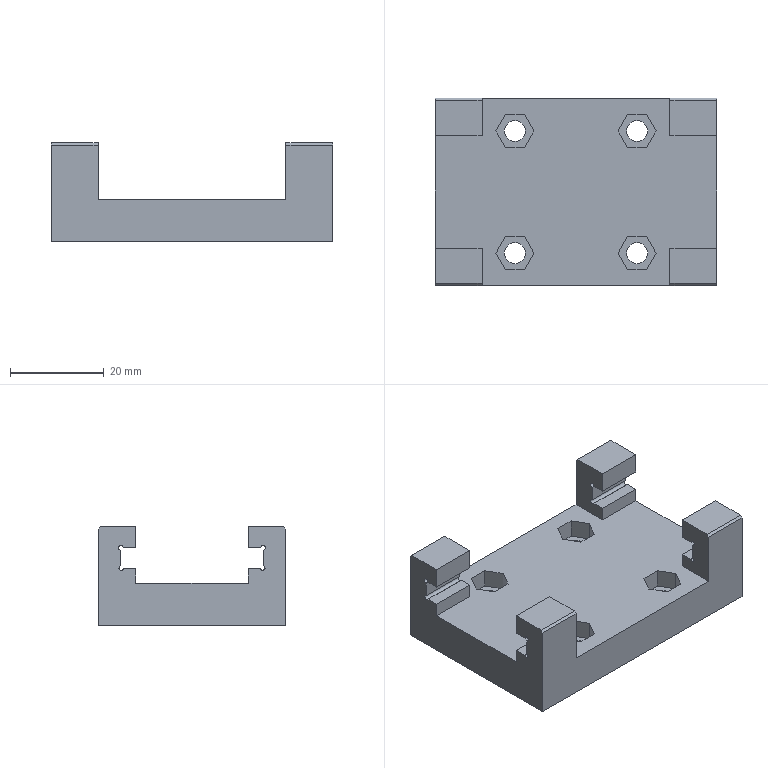Part | SolidWorks | features ICE 6, MirrorPattern 5, Chamfer 1, Extrusion 1 | 1 solid | 86 faces | box 60 x 40 x 21 mm | volume 23831 mm3 | plane 66 | cylinder 20 | commonest cylinder face diameters 1 x12 4.5 x8